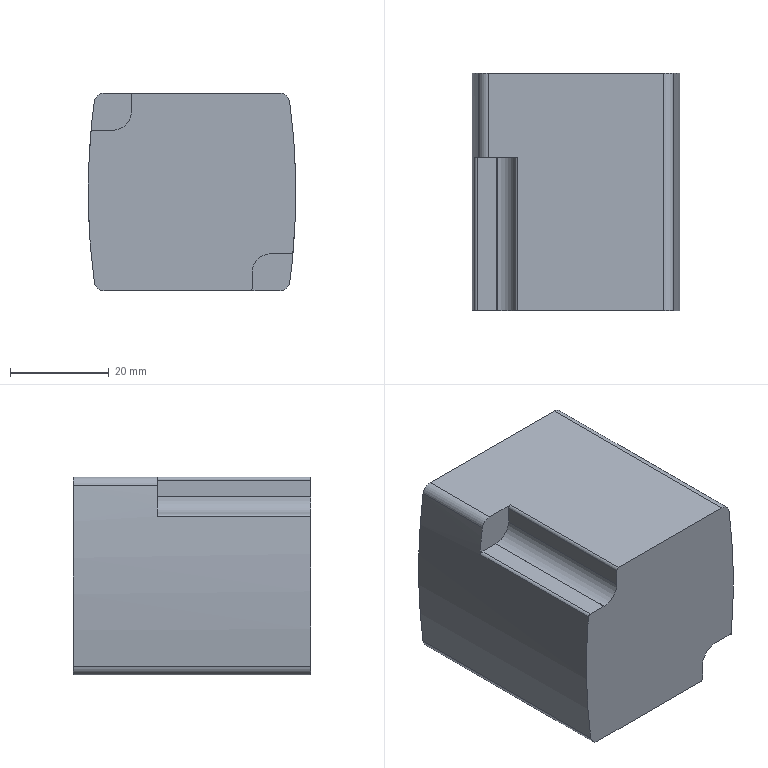Part | SolidWorks | features BaseBody 1 | 1 solid | 27 faces | box 42.009 x 48 x 40 mm | volume 75232 mm3 | cylinder 16 | plane 11 | commonest cylinder face diameters 4 x6 1.2 x5 7.4 x3 268.2 x2
STEP:
#1=CARTESIAN_POINT('',(17.75,48.01,-20.));
#2=VERTEX_POINT('',#1);
#3=CARTESIAN_POINT('',(17.773,48.01,-20.));
#4=VERTEX_POINT('',#3);
#5=CARTESIAN_POINT('',(17.773,48.01,-18.));
#6=DIRECTION('',(0.,-1.,0.));
#7=DIRECTION('',(0.,0.,-1.));
#8=AXIS2_PLACEMENT_3D('',#5,#6,#7);
#9=CIRCLE('',#8,2.);
#10=EDGE_CURVE('',#2,#4,#9,.T.);
#11=ORIENTED_EDGE('',*,*,#10,.T.);
#12=CARTESIAN_POINT('',(17.773,31.01,-20.));
#13=VERTEX_POINT('',#12);
#14=CARTESIAN_POINT('',(17.773,48.01,-20.));
#15=DIRECTION('',(0.,-1.,0.));
#16=VECTOR('',#15,1000.);
#17=LINE('',#14,#16);
#18=EDGE_CURVE('',#4,#13,#17,.T.);
#19=ORIENTED_EDGE('',*,*,#18,.T.);
#20=CARTESIAN_POINT('',(17.75,31.01,-20.));
#21=VERTEX_POINT('',#20);
#22=CARTESIAN_POINT('',(17.773,31.01,-18.));
#23=DIRECTION('',(0.,1.,0.));
#24=DIRECTION('',(0.,0.,-1.));
#25=AXIS2_PLACEMENT_3D('',#22,#23,#24);
#26=CIRCLE('',#25,2.);
#27=EDGE_CURVE('',#13,#21,#26,.T.);
#28=ORIENTED_EDGE('',*,*,#27,.T.);
#29=CARTESIAN_POINT('',(17.75,48.01,-20.));
#30=DIRECTION('',(0.,1.,0.));
#31=VECTOR('',#30,1000.);
#32=LINE('',#29,#31);
#33=EDGE_CURVE('',#21,#2,#32,.T.);
#34=ORIENTED_EDGE('',*,*,#33,.T.);
#35=EDGE_LOOP('',(#11,#19,#28,#34));
#36=FACE_OUTER_BOUND('',#35,.T.);
#37=CARTESIAN_POINT('',(17.773,48.01,-18.));
#38=DIRECTION('',(0.,-1.,0.));
#39=DIRECTION('',(0.,0.,-1.));
#40=AXIS2_PLACEMENT_3D('',#37,#38,#39);
#41=CYLINDRICAL_SURFACE('',#40,2.);
#42=ADVANCED_FACE('',(#36),#41,.T.);
#43=CARTESIAN_POINT('',(-19.75,48.01,-18.3));
#44=VERTEX_POINT('',#43);
#45=CARTESIAN_POINT('',(-17.773,48.01,-20.));
#46=VERTEX_POINT('',#45);
#47=CARTESIAN_POINT('',(-17.773,48.01,-18.));
#48=DIRECTION('',(0.,-1.,0.));
#49=DIRECTION('',(0.,0.,-1.));
#50=AXIS2_PLACEMENT_3D('',#47,#48,#49);
#51=CIRCLE('',#50,2.);
#52=EDGE_CURVE('',#44,#46,#51,.T.);
#53=ORIENTED_EDGE('',*,*,#52,.T.);
#54=CARTESIAN_POINT('',(-17.773,0.01,-20.));
#55=VERTEX_POINT('',#54);
#56=CARTESIAN_POINT('',(-17.773,48.01,-20.));
#57=DIRECTION('',(0.,-1.,0.));
#58=VECTOR('',#57,1000.);
#59=LINE('',#56,#58);
#60=EDGE_CURVE('',#46,#55,#59,.T.);
#61=ORIENTED_EDGE('',*,*,#60,.T.);
#62=CARTESIAN_POINT('',(-19.75,0.01,-18.3));
#63=VERTEX_POINT('',#62);
#64=CARTESIAN_POINT('',(-17.773,0.01,-18.));
#65=DIRECTION('',(0.,1.,0.));
#66=DIRECTION('',(0.,0.,-1.));
#67=AXIS2_PLACEMENT_3D('',#64,#65,#66);
#68=CIRCLE('',#67,2.);
#69=EDGE_CURVE('',#55,#63,#68,.T.);
#70=ORIENTED_EDGE('',*,*,#69,.T.);
#71=CARTESIAN_POINT('',(-19.75,48.01,-18.3));
#72=DIRECTION('',(0.,1.,0.));
#73=VECTOR('',#72,1000.);
#74=LINE('',#71,#73);
#75=EDGE_CURVE('',#63,#44,#74,.T.);
#76=ORIENTED_EDGE('',*,*,#75,.T.);
#77=EDGE_LOOP('',(#53,#61,#70,#76));
#78=FACE_OUTER_BOUND('',#77,.T.);
#79=CARTESIAN_POINT('',(-17.773,48.01,-18.));
#80=DIRECTION('',(0.,-1.,0.));
#81=DIRECTION('',(0.,0.,-1.));
#82=AXIS2_PLACEMENT_3D('',#79,#80,#81);
#83=CYLINDRICAL_SURFACE('',#82,2.);
#84=ADVANCED_FACE('',(#78),#83,.T.);
#85=CARTESIAN_POINT('',(-15.975,31.01,12.51));
#86=VERTEX_POINT('',#85);
#87=CARTESIAN_POINT('',(-12.28,31.01,16.01));
#88=VERTEX_POINT('',#87);
#89=CARTESIAN_POINT('',(-15.975,31.01,16.21));
#90=DIRECTION('',(0.,-1.,0.));
#91=DIRECTION('',(0.,0.,-1.));
#92=AXIS2_PLACEMENT_3D('',#89,#90,#91);
#93=CIRCLE('',#92,3.7);
#94=EDGE_CURVE('',#86,#88,#93,.T.);
#95=ORIENTED_EDGE('',*,*,#94,.F.);
#96=CARTESIAN_POINT('',(-15.975,0.01,12.51));
#97=VERTEX_POINT('',#96);
#98=CARTESIAN_POINT('',(-15.975,31.01,12.51));
#99=DIRECTION('',(0.,-1.,0.));
#100=VECTOR('',#99,1000.);
#101=LINE('',#98,#100);
#102=EDGE_CURVE('',#86,#97,#101,.T.);
#103=ORIENTED_EDGE('',*,*,#102,.T.);
#104=CARTESIAN_POINT('',(-12.28,0.01,16.01));
#105=VERTEX_POINT('',#104);
#106=CARTESIAN_POINT('',(-15.975,0.01,16.21));
#107=DIRECTION('',(0.,1.,0.));
#108=DIRECTION('',(0.,0.,-1.));
#109=AXIS2_PLACEMENT_3D('',#106,#107,#108);
#110=CIRCLE('',#109,3.7);
#111=EDGE_CURVE('',#105,#97,#110,.T.);
#112=ORIENTED_EDGE('',*,*,#111,.F.);
#113=CARTESIAN_POINT('',(-12.28,31.01,16.01));
#114=DIRECTION('',(0.,1.,0.));
#115=VECTOR('',#114,1000.);
#116=LINE('',#113,#115);
#117=EDGE_CURVE('',#105,#88,#116,.T.);
#118=ORIENTED_EDGE('',*,*,#117,.T.);
#119=EDGE_LOOP('',(#95,#103,#112,#118));
#120=FACE_OUTER_BOUND('',#119,.T.);
#121=CARTESIAN_POINT('',(-15.975,31.01,16.21));
#122=DIRECTION('',(0.,-1.,0.));
#123=DIRECTION('',(0.,0.,-1.));
#124=AXIS2_PLACEMENT_3D('',#121,#122,#123);
#125=CYLINDRICAL_SURFACE('',#124,3.7);
#126=ADVANCED_FACE('',(#120),#125,.F.);
#127=CARTESIAN_POINT('',(19.8,31.01,-12.51));
#128=VERTEX_POINT('',#127);
#129=CARTESIAN_POINT('',(19.808,31.01,-12.51));
#130=VERTEX_POINT('',#129);
#131=CARTESIAN_POINT('',(19.808,31.01,-11.91));
#132=DIRECTION('',(0.,-1.,0.));
#133=DIRECTION('',(0.,0.,-1.));
#134=AXIS2_PLACEMENT_3D('',#131,#132,#133);
#135=CIRCLE('',#134,0.6);
#136=EDGE_CURVE('',#128,#130,#135,.T.);
#137=ORIENTED_EDGE('',*,*,#136,.T.);
#138=CARTESIAN_POINT('',(19.808,0.01,-12.51));
#139=VERTEX_POINT('',#138);
#140=CARTESIAN_POINT('',(19.808,31.01,-12.51));
#141=DIRECTION('',(0.,-1.,0.));
#142=VECTOR('',#141,1000.);
#143=LINE('',#140,#142);
#144=EDGE_CURVE('',#130,#139,#143,.T.);
#145=ORIENTED_EDGE('',*,*,#144,.T.);
#146=CARTESIAN_POINT('',(19.8,0.01,-12.51));
#147=VERTEX_POINT('',#146);
#148=CARTESIAN_POINT('',(19.808,0.01,-11.91));
#149=DIRECTION('',(0.,1.,0.));
#150=DIRECTION('',(0.,0.,-1.));
#151=AXIS2_PLACEMENT_3D('',#148,#149,#150);
#152=CIRCLE('',#151,0.6);
#153=EDGE_CURVE('',#139,#147,#152,.T.);
#154=ORIENTED_EDGE('',*,*,#153,.T.);
#155=CARTESIAN_POINT('',(19.8,31.01,-12.51));
#156=DIRECTION('',(0.,1.,0.));
#157=VECTOR('',#156,1000.);
#158=LINE('',#155,#157);
#159=EDGE_CURVE('',#147,#128,#158,.T.);
#160=ORIENTED_EDGE('',*,*,#159,.T.);
#161=EDGE_LOOP('',(#137,#145,#154,#160));
#162=FACE_OUTER_BOUND('',#161,.T.);
#163=CARTESIAN_POINT('',(19.808,31.01,-11.91));
#164=DIRECTION('',(0.,-1.,0.));
#165=DIRECTION('',(0.,0.,-1.));
#166=AXIS2_PLACEMENT_3D('',#163,#164,#165);
#167=CYLINDRICAL_SURFACE('',#166,0.6);
#168=ADVANCED_FACE('',(#162),#167,.T.);
#169=CARTESIAN_POINT('',(19.75,48.01,18.3));
#170=VERTEX_POINT('',#169);
#171=CARTESIAN_POINT('',(17.75,48.01,20.));
#172=VERTEX_POINT('',#171);
#173=CARTESIAN_POINT('',(17.773,48.01,18.));
#174=DIRECTION('',(0.,-1.,0.));
#175=DIRECTION('',(0.,0.,-1.));
#176=AXIS2_PLACEMENT_3D('',#173,#174,#175);
#177=CIRCLE('',#176,2.);
#178=EDGE_CURVE('',#170,#172,#177,.T.);
#179=ORIENTED_EDGE('',*,*,#178,.F.);
#180=CARTESIAN_POINT('',(19.75,48.01,-18.3));
#181=VERTEX_POINT('',#180);
#182=CARTESIAN_POINT('',(-113.095,48.01,0.));
#183=DIRECTION('',(0.,-1.,0.));
#184=DIRECTION('',(0.,0.,-1.));
#185=AXIS2_PLACEMENT_3D('',#182,#183,#184);
#186=CIRCLE('',#185,134.1);
#187=EDGE_CURVE('',#181,#170,#186,.T.);
#188=ORIENTED_EDGE('',*,*,#187,.F.);
#189=CARTESIAN_POINT('',(17.773,48.01,-18.));
#190=DIRECTION('',(0.,-1.,0.));
#191=DIRECTION('',(0.,0.,-1.));
#192=AXIS2_PLACEMENT_3D('',#189,#190,#191);
#193=CIRCLE('',#192,2.);
#194=EDGE_CURVE('',#4,#181,#193,.T.);
#195=ORIENTED_EDGE('',*,*,#194,.F.);
#196=ORIENTED_EDGE('',*,*,#10,.F.);
#197=CARTESIAN_POINT('',(-17.75,48.01,-20.));
#198=VERTEX_POINT('',#197);
#199=CARTESIAN_POINT('',(0.,48.01,-20.));
#200=DIRECTION('',(1.,0.,0.));
#201=VECTOR('',#200,1000.);
#202=LINE('',#199,#201);
#203=EDGE_CURVE('',#198,#2,#202,.T.);
#204=ORIENTED_EDGE('',*,*,#203,.F.);
#205=CARTESIAN_POINT('',(-17.773,48.01,-18.));
#206=DIRECTION('',(0.,-1.,0.));
#207=DIRECTION('',(0.,0.,-1.));
#208=AXIS2_PLACEMENT_3D('',#205,#206,#207);
#209=CIRCLE('',#208,2.);
#210=EDGE_CURVE('',#46,#198,#209,.T.);
#211=ORIENTED_EDGE('',*,*,#210,.F.);
#212=ORIENTED_EDGE('',*,*,#52,.F.);
#213=CARTESIAN_POINT('',(-19.75,48.01,18.3));
#214=VERTEX_POINT('',#213);
#215=CARTESIAN_POINT('',(113.095,48.01,0.));
#216=DIRECTION('',(0.,-1.,0.));
#217=DIRECTION('',(0.,0.,-1.));
#218=AXIS2_PLACEMENT_3D('',#215,#216,#217);
#219=CIRCLE('',#218,134.1);
#220=EDGE_CURVE('',#214,#44,#219,.T.);
#221=ORIENTED_EDGE('',*,*,#220,.F.);
#222=CARTESIAN_POINT('',(-17.75,48.01,20.));
#223=VERTEX_POINT('',#222);
#224=CARTESIAN_POINT('',(-17.773,48.01,18.));
#225=DIRECTION('',(0.,-1.,0.));
#226=DIRECTION('',(0.,0.,-1.));
#227=AXIS2_PLACEMENT_3D('',#224,#225,#226);
#228=CIRCLE('',#227,2.);
#229=EDGE_CURVE('',#223,#214,#228,.T.);
#230=ORIENTED_EDGE('',*,*,#229,.F.);
#231=CARTESIAN_POINT('',(0.,48.01,20.));
#232=DIRECTION('',(-1.,0.,0.));
#233=VECTOR('',#232,1000.);
#234=LINE('',#231,#233);
#235=EDGE_CURVE('',#172,#223,#234,.T.);
#236=ORIENTED_EDGE('',*,*,#235,.F.);
#237=EDGE_LOOP('',(#179,#188,#195,#196,#204,#211,#212,#221,#230,#236));
#238=FACE_OUTER_BOUND('',#237,.T.);
#239=CARTESIAN_POINT('',(0.,48.01,0.));
#240=DIRECTION('',(0.,-1.,0.));
#241=DIRECTION('',(0.,0.,-1.));
#242=AXIS2_PLACEMENT_3D('',#239,#240,#241);
#243=PLANE('',#242);
#244=ADVANCED_FACE('',(#238),#243,.F.);
#245=CARTESIAN_POINT('',(-17.75,31.01,20.));
#246=VERTEX_POINT('',#245);
#247=CARTESIAN_POINT('',(-17.75,48.01,20.));
#248=DIRECTION('',(0.,-1.,0.));
#249=VECTOR('',#248,1000.);
#250=LINE('',#247,#249);
#251=EDGE_CURVE('',#223,#246,#250,.T.);
#252=ORIENTED_EDGE('',*,*,#251,.T.);
#253=CARTESIAN_POINT('',(-11.789,31.01,20.));
#254=VERTEX_POINT('',#253);
#255=CARTESIAN_POINT('',(8.875,31.01,20.));
#256=DIRECTION('',(1.,0.,0.));
#257=VECTOR('',#256,1000.);
#258=LINE('',#255,#257);
#259=EDGE_CURVE('',#246,#254,#258,.T.);
#260=ORIENTED_EDGE('',*,*,#259,.T.);
#261=CARTESIAN_POINT('',(-11.789,0.01,20.));
#262=VERTEX_POINT('',#261);
#263=CARTESIAN_POINT('',(-11.789,48.01,20.));
#264=DIRECTION('',(0.,-1.,0.));
#265=VECTOR('',#264,1000.);
#266=LINE('',#263,#265);
#267=EDGE_CURVE('',#254,#262,#266,.T.);
#268=ORIENTED_EDGE('',*,*,#267,.T.);
#269=CARTESIAN_POINT('',(17.75,0.01,20.));
#270=VERTEX_POINT('',#269);
#271=CARTESIAN_POINT('',(8.875,0.01,20.));
#272=DIRECTION('',(1.,0.,0.));
#273=VECTOR('',#272,1000.);
#274=LINE('',#271,#273);
#275=EDGE_CURVE('',#262,#270,#274,.T.);
#276=ORIENTED_EDGE('',*,*,#275,.T.);
#277=CARTESIAN_POINT('',(17.75,48.01,20.));
#278=DIRECTION('',(0.,1.,0.));
#279=VECTOR('',#278,1000.);
#280=LINE('',#277,#279);
#281=EDGE_CURVE('',#270,#172,#280,.T.);
#282=ORIENTED_EDGE('',*,*,#281,.T.);
#283=ORIENTED_EDGE('',*,*,#235,.T.);
#284=EDGE_LOOP('',(#252,#260,#268,#276,#282,#283));
#285=FACE_OUTER_BOUND('',#284,.T.);
#286=CARTESIAN_POINT('',(8.875,48.01,20.));
#287=DIRECTION('',(0.,0.,1.));
#288=DIRECTION('',(1.,0.,0.));
#289=AXIS2_PLACEMENT_3D('',#286,#287,#288);
#290=PLANE('',#289);
#291=ADVANCED_FACE('',(#285),#290,.T.);
#292=ORIENTED_EDGE('',*,*,#178,.T.);
#293=ORIENTED_EDGE('',*,*,#281,.F.);
#294=CARTESIAN_POINT('',(19.75,0.01,18.3));
#295=VERTEX_POINT('',#294);
#296=CARTESIAN_POINT('',(17.773,0.01,18.));
#297=DIRECTION('',(0.,1.,0.));
#298=DIRECTION('',(0.,0.,-1.));
#299=AXIS2_PLACEMENT_3D('',#296,#297,#298);
#300=CIRCLE('',#299,2.);
#301=EDGE_CURVE('',#270,#295,#300,.T.);
#302=ORIENTED_EDGE('',*,*,#301,.T.);
#303=CARTESIAN_POINT('',(19.75,48.01,18.3));
#304=DIRECTION('',(0.,1.,0.));
#305=VECTOR('',#304,1000.);
#306=LINE('',#303,#305);
#307=EDGE_CURVE('',#295,#170,#306,.T.);
#308=ORIENTED_EDGE('',*,*,#307,.T.);
#309=EDGE_LOOP('',(#292,#293,#302,#308));
#310=FACE_OUTER_BOUND('',#309,.T.);
#311=CARTESIAN_POINT('',(17.773,48.01,18.));
#312=DIRECTION('',(0.,-1.,0.));
#313=DIRECTION('',(0.,0.,-1.));
#314=AXIS2_PLACEMENT_3D('',#311,#312,#313);
#315=CYLINDRICAL_SURFACE('',#314,2.);
#316=ADVANCED_FACE('',(#310),#315,.T.);
#317=ORIENTED_EDGE('',*,*,#307,.F.);
#318=CARTESIAN_POINT('',(20.4,0.01,-12.719));
#319=VERTEX_POINT('',#318);
#320=CARTESIAN_POINT('',(-113.095,0.01,0.));
#321=DIRECTION('',(0.,1.,0.));
#322=DIRECTION('',(0.,0.,-1.));
#323=AXIS2_PLACEMENT_3D('',#320,#321,#322);
#324=CIRCLE('',#323,134.1);
#325=EDGE_CURVE('',#295,#319,#324,.T.);
#326=ORIENTED_EDGE('',*,*,#325,.T.);
#327=CARTESIAN_POINT('',(20.4,31.01,-12.719));
#328=VERTEX_POINT('',#327);
#329=CARTESIAN_POINT('',(20.4,48.01,-12.719));
#330=DIRECTION('',(0.,1.,0.));
#331=VECTOR('',#330,1000.);
#332=LINE('',#329,#331);
#333=EDGE_CURVE('',#319,#328,#332,.T.);
#334=ORIENTED_EDGE('',*,*,#333,.T.);
#335=CARTESIAN_POINT('',(19.75,31.01,-18.3));
#336=VERTEX_POINT('',#335);
#337=CARTESIAN_POINT('',(-113.095,31.01,0.));
#338=DIRECTION('',(0.,1.,0.));
#339=DIRECTION('',(0.,0.,-1.));
#340=AXIS2_PLACEMENT_3D('',#337,#338,#339);
#341=CIRCLE('',#340,134.1);
#342=EDGE_CURVE('',#328,#336,#341,.T.);
#343=ORIENTED_EDGE('',*,*,#342,.T.);
#344=CARTESIAN_POINT('',(19.75,48.01,-18.3));
#345=DIRECTION('',(0.,1.,0.));
#346=VECTOR('',#345,1000.);
#347=LINE('',#344,#346);
#348=EDGE_CURVE('',#336,#181,#347,.T.);
#349=ORIENTED_EDGE('',*,*,#348,.T.);
#350=ORIENTED_EDGE('',*,*,#187,.T.);
#351=EDGE_LOOP('',(#317,#326,#334,#343,#349,#350));
#352=FACE_OUTER_BOUND('',#351,.T.);
#353=CARTESIAN_POINT('',(-113.095,48.01,0.));
#354=DIRECTION('',(0.,-1.,0.));
#355=DIRECTION('',(0.,0.,-1.));
#356=AXIS2_PLACEMENT_3D('',#353,#354,#355);
#357=CYLINDRICAL_SURFACE('',#356,134.1);
#358=ADVANCED_FACE('',(#352),#357,.T.);
#359=ORIENTED_EDGE('',*,*,#18,.F.);
#360=ORIENTED_EDGE('',*,*,#194,.T.);
#361=ORIENTED_EDGE('',*,*,#348,.F.);
#362=CARTESIAN_POINT('',(17.773,31.01,-18.));
#363=DIRECTION('',(0.,1.,0.));
#364=DIRECTION('',(0.,0.,-1.));
#365=AXIS2_PLACEMENT_3D('',#362,#363,#364);
#366=CIRCLE('',#365,2.);
#367=EDGE_CURVE('',#336,#13,#366,.T.);
#368=ORIENTED_EDGE('',*,*,#367,.T.);
#369=EDGE_LOOP('',(#359,#360,#361,#368));
#370=FACE_OUTER_BOUND('',#369,.T.);
#371=CARTESIAN_POINT('',(17.773,48.01,-18.));
#372=DIRECTION('',(0.,-1.,0.));
#373=DIRECTION('',(0.,0.,-1.));
#374=AXIS2_PLACEMENT_3D('',#371,#372,#373);
#375=CYLINDRICAL_SURFACE('',#374,2.);
#376=ADVANCED_FACE('',(#370),#375,.T.);
#377=ORIENTED_EDGE('',*,*,#203,.T.);
#378=ORIENTED_EDGE('',*,*,#33,.F.);
#379=CARTESIAN_POINT('',(11.709,31.01,-20.));
#380=VERTEX_POINT('',#379);
#381=CARTESIAN_POINT('',(0.,31.01,-20.));
#382=DIRECTION('',(-1.,0.,0.));
#383=VECTOR('',#382,1000.);
#384=LINE('',#381,#383);
#385=EDGE_CURVE('',#21,#380,#384,.T.);
#386=ORIENTED_EDGE('',*,*,#385,.T.);
#387=CARTESIAN_POINT('',(11.709,0.01,-20.));
#388=VERTEX_POINT('',#387);
#389=CARTESIAN_POINT('',(11.709,48.01,-20.));
#390=DIRECTION('',(0.,-1.,0.));
#391=VECTOR('',#390,1000.);
#392=LINE('',#389,#391);
#393=EDGE_CURVE('',#380,#388,#392,.T.);
#394=ORIENTED_EDGE('',*,*,#393,.T.);
#395=CARTESIAN_POINT('',(-17.75,0.01,-20.));
#396=VERTEX_POINT('',#395);
#397=CARTESIAN_POINT('',(0.,0.01,-20.));
#398=DIRECTION('',(-1.,0.,0.));
#399=VECTOR('',#398,1000.);
#400=LINE('',#397,#399);
#401=EDGE_CURVE('',#388,#396,#400,.T.);
#402=ORIENTED_EDGE('',*,*,#401,.T.);
#403=CARTESIAN_POINT('',(-17.75,48.01,-20.));
#404=DIRECTION('',(0.,1.,0.));
#405=VECTOR('',#404,1000.);
#406=LINE('',#403,#405);
#407=EDGE_CURVE('',#396,#198,#406,.T.);
#408=ORIENTED_EDGE('',*,*,#407,.T.);
#409=EDGE_LOOP('',(#377,#378,#386,#394,#402,#408));
#410=FACE_OUTER_BOUND('',#409,.T.);
#411=CARTESIAN_POINT('',(0.,48.01,-20.));
#412=DIRECTION('',(0.,0.,-1.));
#413=DIRECTION('',(-1.,0.,0.));
#414=AXIS2_PLACEMENT_3D('',#411,#412,#413);
#415=PLANE('',#414);
#416=ADVANCED_FACE('',(#410),#415,.T.);
#417=ORIENTED_EDGE('',*,*,#60,.F.);
#418=ORIENTED_EDGE('',*,*,#210,.T.);
#419=ORIENTED_EDGE('',*,*,#407,.F.);
#420=CARTESIAN_POINT('',(-17.773,0.01,-18.));
#421=DIRECTION('',(0.,1.,0.));
#422=DIRECTION('',(0.,0.,-1.));
#423=AXIS2_PLACEMENT_3D('',#420,#421,#422);
#424=CIRCLE('',#423,2.);
#425=EDGE_CURVE('',#396,#55,#424,.T.);
#426=ORIENTED_EDGE('',*,*,#425,.T.);
#427=EDGE_LOOP('',(#417,#418,#419,#426));
#428=FACE_OUTER_BOUND('',#427,.T.);
#429=CARTESIAN_POINT('',(-17.773,48.01,-18.));
#430=DIRECTION('',(0.,-1.,0.));
#431=DIRECTION('',(0.,0.,-1.));
#432=AXIS2_PLACEMENT_3D('',#429,#430,#431);
#433=CYLINDRICAL_SURFACE('',#432,2.);
#434=ADVANCED_FACE('',(#428),#433,.T.);
#435=CARTESIAN_POINT('',(-20.458,0.01,12.1));
#436=VERTEX_POINT('',#435);
#437=CARTESIAN_POINT('',(113.095,0.01,0.));
#438=DIRECTION('',(0.,1.,0.));
#439=DIRECTION('',(0.,0.,-1.));
#440=AXIS2_PLACEMENT_3D('',#437,#438,#439);
#441=CIRCLE('',#440,134.1);
#442=EDGE_CURVE('',#63,#436,#441,.T.);
#443=ORIENTED_EDGE('',*,*,#442,.T.);
#444=CARTESIAN_POINT('',(-20.458,31.01,12.1));
#445=VERTEX_POINT('',#444);
#446=CARTESIAN_POINT('',(-20.458,48.01,12.1));
#447=DIRECTION('',(0.,1.,0.));
#448=VECTOR('',#447,1000.);
#449=LINE('',#446,#448);
#450=EDGE_CURVE('',#436,#445,#449,.T.);
#451=ORIENTED_EDGE('',*,*,#450,.T.);
#452=CARTESIAN_POINT('',(-19.75,31.01,18.3));
#453=VERTEX_POINT('',#452);
#454=CARTESIAN_POINT('',(113.095,31.01,0.));
#455=DIRECTION('',(0.,1.,0.));
#456=DIRECTION('',(0.,0.,-1.));
#457=AXIS2_PLACEMENT_3D('',#454,#455,#456);
#458=CIRCLE('',#457,134.1);
#459=EDGE_CURVE('',#445,#453,#458,.T.);
#460=ORIENTED_EDGE('',*,*,#459,.T.);
#461=CARTESIAN_POINT('',(-19.75,48.01,18.3));
#462=DIRECTION('',(0.,1.,0.));
#463=VECTOR('',#462,1000.);
#464=LINE('',#461,#463);
#465=EDGE_CURVE('',#453,#214,#464,.T.);
#466=ORIENTED_EDGE('',*,*,#465,.T.);
#467=ORIENTED_EDGE('',*,*,#220,.T.);
#468=ORIENTED_EDGE('',*,*,#75,.F.);
#469=EDGE_LOOP('',(#443,#451,#460,#466,#467,#468));
#470=FACE_OUTER_BOUND('',#469,.T.);
#471=CARTESIAN_POINT('',(113.095,48.01,0.));
#472=DIRECTION('',(0.,-1.,0.));
#473=DIRECTION('',(0.,0.,-1.));
#474=AXIS2_PLACEMENT_3D('',#471,#472,#473);
#475=CYLINDRICAL_SURFACE('',#474,134.1);
#476=ADVANCED_FACE('',(#470),#475,.T.);
#477=ORIENTED_EDGE('',*,*,#229,.T.);
#478=ORIENTED_EDGE('',*,*,#465,.F.);
#479=CARTESIAN_POINT('',(-17.773,31.01,18.));
#480=DIRECTION('',(0.,1.,0.));
#481=DIRECTION('',(0.,0.,-1.));
#482=AXIS2_PLACEMENT_3D('',#479,#480,#481);
#483=CIRCLE('',#482,2.);
#484=EDGE_CURVE('',#453,#246,#483,.T.);
#485=ORIENTED_EDGE('',*,*,#484,.T.);
#486=ORIENTED_EDGE('',*,*,#251,.F.);
#487=EDGE_LOOP('',(#477,#478,#485,#486));
#488=FACE_OUTER_BOUND('',#487,.T.);
#489=CARTESIAN_POINT('',(-17.773,48.01,18.));
#490=DIRECTION('',(0.,-1.,0.));
#491=DIRECTION('',(0.,0.,-1.));
#492=AXIS2_PLACEMENT_3D('',#489,#490,#491);
#493=CYLINDRICAL_SURFACE('',#492,2.);
#494=ADVANCED_FACE('',(#488),#493,.T.);
#495=CARTESIAN_POINT('',(-12.28,31.01,19.41));
#496=VERTEX_POINT('',#495);
#497=CARTESIAN_POINT('',(-12.28,31.01,16.501));
#498=DIRECTION('',(0.,0.,1.));
#499=VECTOR('',#498,1000.);
#500=LINE('',#497,#499);
#501=EDGE_CURVE('',#88,#496,#500,.T.);
#502=ORIENTED_EDGE('',*,*,#501,.T.);
#503=CARTESIAN_POINT('',(-11.68,31.01,19.41));
#504=DIRECTION('',(0.,1.,0.));
#505=DIRECTION('',(0.,0.,-1.));
#506=AXIS2_PLACEMENT_3D('',#503,#504,#505);
#507=CIRCLE('',#506,0.6);
#508=EDGE_CURVE('',#496,#254,#507,.T.);
#509=ORIENTED_EDGE('',*,*,#508,.T.);
#510=ORIENTED_EDGE('',*,*,#259,.F.);
#511=ORIENTED_EDGE('',*,*,#484,.F.);
#512=ORIENTED_EDGE('',*,*,#459,.F.);
#513=CARTESIAN_POINT('',(-19.88,31.01,12.51));
#514=VERTEX_POINT('',#513);
#515=CARTESIAN_POINT('',(-19.888,31.01,11.91));
#516=DIRECTION('',(0.,1.,0.));
#517=DIRECTION('',(0.,0.,-1.));
#518=AXIS2_PLACEMENT_3D('',#515,#516,#517);
#519=CIRCLE('',#518,0.6);
#520=EDGE_CURVE('',#445,#514,#519,.T.);
#521=ORIENTED_EDGE('',*,*,#520,.T.);
#522=CARTESIAN_POINT('',(-15.98,31.01,12.51));
#523=VERTEX_POINT('',#522);
#524=CARTESIAN_POINT('',(-16.586,31.01,12.51));
#525=DIRECTION('',(1.,0.,0.));
#526=VECTOR('',#525,1000.);
#527=LINE('',#524,#526);
#528=EDGE_CURVE('',#514,#523,#527,.T.);
#529=ORIENTED_EDGE('',*,*,#528,.T.);
#530=CARTESIAN_POINT('',(-15.975,31.01,16.21));
#531=DIRECTION('',(0.,-1.,0.));
#532=DIRECTION('',(0.,0.,-1.));
#533=AXIS2_PLACEMENT_3D('',#530,#531,#532);
#534=CIRCLE('',#533,3.7);
#535=EDGE_CURVE('',#523,#86,#534,.T.);
#536=ORIENTED_EDGE('',*,*,#535,.T.);
#537=ORIENTED_EDGE('',*,*,#94,.T.);
#538=EDGE_LOOP('',(#502,#509,#510,#511,#512,#521,#529,#536,#537));
#539=FACE_OUTER_BOUND('',#538,.T.);
#540=CARTESIAN_POINT('',(-16.586,31.01,16.501));
#541=DIRECTION('',(0.,-1.,0.));
#542=DIRECTION('',(0.,0.,-1.));
#543=AXIS2_PLACEMENT_3D('',#540,#541,#542);
#544=PLANE('',#543);
#545=ADVANCED_FACE('',(#539),#544,.T.);
#546=CARTESIAN_POINT('',(15.9,0.01,-12.51));
#547=VERTEX_POINT('',#546);
#548=CARTESIAN_POINT('',(0.,0.01,-12.51));
#549=DIRECTION('',(1.,0.,0.));
#550=VECTOR('',#549,1000.);
#551=LINE('',#548,#550);
#552=EDGE_CURVE('',#547,#147,#551,.T.);
#553=ORIENTED_EDGE('',*,*,#552,.T.);
#554=ORIENTED_EDGE('',*,*,#153,.F.);
#555=CARTESIAN_POINT('',(20.4,0.01,-12.01));
#556=VERTEX_POINT('',#555);
#557=CARTESIAN_POINT('',(19.808,0.01,-11.91));
#558=DIRECTION('',(0.,1.,0.));
#559=DIRECTION('',(0.,0.,-1.));
#560=AXIS2_PLACEMENT_3D('',#557,#558,#559);
#561=CIRCLE('',#560,0.6);
#562=EDGE_CURVE('',#556,#139,#561,.T.);
#563=ORIENTED_EDGE('',*,*,#562,.F.);
#564=CARTESIAN_POINT('',(20.4,0.01,0.));
#565=DIRECTION('',(0.,0.,-1.));
#566=VECTOR('',#565,1000.);
#567=LINE('',#564,#566);
#568=EDGE_CURVE('',#556,#319,#567,.T.);
#569=ORIENTED_EDGE('',*,*,#568,.T.);
#570=ORIENTED_EDGE('',*,*,#325,.F.);
#571=ORIENTED_EDGE('',*,*,#301,.F.);
#572=ORIENTED_EDGE('',*,*,#275,.F.);
#573=CARTESIAN_POINT('',(-12.28,0.01,19.41));
#574=VERTEX_POINT('',#573);
#575=CARTESIAN_POINT('',(-11.68,0.01,19.41));
#576=DIRECTION('',(0.,-1.,0.));
#577=DIRECTION('',(0.,0.,-1.));
#578=AXIS2_PLACEMENT_3D('',#575,#576,#577);
#579=CIRCLE('',#578,0.6);
#580=EDGE_CURVE('',#262,#574,#579,.T.);
#581=ORIENTED_EDGE('',*,*,#580,.T.);
#582=CARTESIAN_POINT('',(-12.28,0.01,0.));
#583=DIRECTION('',(0.,0.,-1.));
#584=VECTOR('',#583,1000.);
#585=LINE('',#582,#584);
#586=EDGE_CURVE('',#574,#105,#585,.T.);
#587=ORIENTED_EDGE('',*,*,#586,.T.);
#588=ORIENTED_EDGE('',*,*,#111,.T.);
#589=CARTESIAN_POINT('',(-15.98,0.01,12.51));
#590=VERTEX_POINT('',#589);
#591=CARTESIAN_POINT('',(-15.975,0.01,16.21));
#592=DIRECTION('',(0.,1.,0.));
#593=DIRECTION('',(0.,0.,-1.));
#594=AXIS2_PLACEMENT_3D('',#591,#592,#593);
#595=CIRCLE('',#594,3.7);
#596=EDGE_CURVE('',#97,#590,#595,.T.);
#597=ORIENTED_EDGE('',*,*,#596,.T.);
#598=CARTESIAN_POINT('',(-19.88,0.01,12.51));
#599=VERTEX_POINT('',#598);
#600=CARTESIAN_POINT('',(0.,0.01,12.51));
#601=DIRECTION('',(-1.,0.,0.));
#602=VECTOR('',#601,1000.);
#603=LINE('',#600,#602);
#604=EDGE_CURVE('',#590,#599,#603,.T.);
#605=ORIENTED_EDGE('',*,*,#604,.T.);
#606=CARTESIAN_POINT('',(-19.888,0.01,11.91));
#607=DIRECTION('',(0.,-1.,0.));
#608=DIRECTION('',(0.,0.,-1.));
#609=AXIS2_PLACEMENT_3D('',#606,#607,#608);
#610=CIRCLE('',#609,0.6);
#611=EDGE_CURVE('',#599,#436,#610,.T.);
#612=ORIENTED_EDGE('',*,*,#611,.T.);
#613=ORIENTED_EDGE('',*,*,#442,.F.);
#614=ORIENTED_EDGE('',*,*,#69,.F.);
#615=ORIENTED_EDGE('',*,*,#425,.F.);
#616=ORIENTED_EDGE('',*,*,#401,.F.);
#617=CARTESIAN_POINT('',(12.2,0.01,-19.41));
#618=VERTEX_POINT('',#617);
#619=CARTESIAN_POINT('',(11.6,0.01,-19.41));
#620=DIRECTION('',(0.,-1.,0.));
#621=DIRECTION('',(0.,0.,-1.));
#622=AXIS2_PLACEMENT_3D('',#619,#620,#621);
#623=CIRCLE('',#622,0.6);
#624=EDGE_CURVE('',#388,#618,#623,.T.);
#625=ORIENTED_EDGE('',*,*,#624,.T.);
#626=CARTESIAN_POINT('',(12.2,0.01,-16.01));
#627=VERTEX_POINT('',#626);
#628=CARTESIAN_POINT('',(12.2,0.01,0.));
#629=DIRECTION('',(0.,0.,1.));
#630=VECTOR('',#629,1000.);
#631=LINE('',#628,#630);
#632=EDGE_CURVE('',#618,#627,#631,.T.);
#633=ORIENTED_EDGE('',*,*,#632,.T.);
#634=CARTESIAN_POINT('',(15.895,0.01,-16.21));
#635=DIRECTION('',(0.,1.,0.));
#636=DIRECTION('',(0.,0.,-1.));
#637=AXIS2_PLACEMENT_3D('',#634,#635,#636);
#638=CIRCLE('',#637,3.7);
#639=EDGE_CURVE('',#627,#547,#638,.T.);
#640=ORIENTED_EDGE('',*,*,#639,.T.);
#641=EDGE_LOOP('',(#553,#554,#563,#569,#570,#571,#572,#581,#587,#588,#597,#605,#612,#613,#614,#615,#616,#625,#633,#640));
#642=FACE_OUTER_BOUND('',#641,.T.);
#643=CARTESIAN_POINT('',(0.,0.01,0.));
#644=DIRECTION('',(0.,-1.,0.));
#645=DIRECTION('',(0.,0.,-1.));
#646=AXIS2_PLACEMENT_3D('',#643,#644,#645);
#647=PLANE('',#646);
#648=ADVANCED_FACE('',(#642),#647,.T.);
#649=CARTESIAN_POINT('',(-12.28,31.01,19.41));
#650=DIRECTION('',(0.,-1.,0.));
#651=VECTOR('',#650,1000.);
#652=LINE('',#649,#651);
#653=EDGE_CURVE('',#496,#574,#652,.T.);
#654=ORIENTED_EDGE('',*,*,#653,.T.);
#655=ORIENTED_EDGE('',*,*,#580,.F.);
#656=ORIENTED_EDGE('',*,*,#267,.F.);
#657=ORIENTED_EDGE('',*,*,#508,.F.);
#658=EDGE_LOOP('',(#654,#655,#656,#657));
#659=FACE_OUTER_BOUND('',#658,.T.);
#660=CARTESIAN_POINT('',(-11.68,31.01,19.41));
#661=DIRECTION('',(0.,-1.,0.));
#662=DIRECTION('',(0.,0.,-1.));
#663=AXIS2_PLACEMENT_3D('',#660,#661,#662);
#664=CYLINDRICAL_SURFACE('',#663,0.6);
#665=ADVANCED_FACE('',(#659),#664,.T.);
#666=ORIENTED_EDGE('',*,*,#385,.F.);
#667=ORIENTED_EDGE('',*,*,#27,.F.);
#668=ORIENTED_EDGE('',*,*,#367,.F.);
#669=ORIENTED_EDGE('',*,*,#342,.F.);
#670=CARTESIAN_POINT('',(20.4,31.01,-12.01));
#671=VERTEX_POINT('',#670);
#672=CARTESIAN_POINT('',(20.4,31.01,-16.501));
#673=DIRECTION('',(0.,0.,1.));
#674=VECTOR('',#673,1000.);
#675=LINE('',#672,#674);
#676=EDGE_CURVE('',#328,#671,#675,.T.);
#677=ORIENTED_EDGE('',*,*,#676,.T.);
#678=CARTESIAN_POINT('',(19.808,31.01,-11.91));
#679=DIRECTION('',(0.,-1.,0.));
#680=DIRECTION('',(0.,0.,-1.));
#681=AXIS2_PLACEMENT_3D('',#678,#679,#680);
#682=CIRCLE('',#681,0.6);
#683=EDGE_CURVE('',#130,#671,#682,.T.);
#684=ORIENTED_EDGE('',*,*,#683,.F.);
#685=ORIENTED_EDGE('',*,*,#136,.F.);
#686=CARTESIAN_POINT('',(15.9,31.01,-12.51));
#687=VERTEX_POINT('',#686);
#688=CARTESIAN_POINT('',(16.506,31.01,-12.51));
#689=DIRECTION('',(-1.,0.,0.));
#690=VECTOR('',#689,1000.);
#691=LINE('',#688,#690);
#692=EDGE_CURVE('',#128,#687,#691,.T.);
#693=ORIENTED_EDGE('',*,*,#692,.T.);
#694=CARTESIAN_POINT('',(12.2,31.01,-16.01));
#695=VERTEX_POINT('',#694);
#696=CARTESIAN_POINT('',(15.895,31.01,-16.21));
#697=DIRECTION('',(0.,-1.,0.));
#698=DIRECTION('',(0.,0.,-1.));
#699=AXIS2_PLACEMENT_3D('',#696,#697,#698);
#700=CIRCLE('',#699,3.7);
#701=EDGE_CURVE('',#687,#695,#700,.T.);
#702=ORIENTED_EDGE('',*,*,#701,.T.);
#703=CARTESIAN_POINT('',(12.2,31.01,-19.41));
#704=VERTEX_POINT('',#703);
#705=CARTESIAN_POINT('',(12.2,31.01,-16.501));
#706=DIRECTION('',(0.,0.,-1.));
#707=VECTOR('',#706,1000.);
#708=LINE('',#705,#707);
#709=EDGE_CURVE('',#695,#704,#708,.T.);
#710=ORIENTED_EDGE('',*,*,#709,.T.);
#711=CARTESIAN_POINT('',(11.6,31.01,-19.41));
#712=DIRECTION('',(0.,1.,0.));
#713=DIRECTION('',(0.,0.,-1.));
#714=AXIS2_PLACEMENT_3D('',#711,#712,#713);
#715=CIRCLE('',#714,0.6);
#716=EDGE_CURVE('',#704,#380,#715,.T.);
#717=ORIENTED_EDGE('',*,*,#716,.T.);
#718=EDGE_LOOP('',(#666,#667,#668,#669,#677,#684,#685,#693,#702,#710,#717));
#719=FACE_OUTER_BOUND('',#718,.T.);
#720=CARTESIAN_POINT('',(16.506,31.01,-16.501));
#721=DIRECTION('',(0.,-1.,0.));
#722=DIRECTION('',(0.,0.,-1.));
#723=AXIS2_PLACEMENT_3D('',#720,#721,#722);
#724=PLANE('',#723);
#725=ADVANCED_FACE('',(#719),#724,.T.);
#726=ORIENTED_EDGE('',*,*,#568,.F.);
#727=CARTESIAN_POINT('',(20.4,31.01,-12.01));
#728=DIRECTION('',(0.,-1.,0.));
#729=VECTOR('',#728,1000.);
#730=LINE('',#727,#729);
#731=EDGE_CURVE('',#671,#556,#730,.T.);
#732=ORIENTED_EDGE('',*,*,#731,.F.);
#733=ORIENTED_EDGE('',*,*,#676,.F.);
#734=ORIENTED_EDGE('',*,*,#333,.F.);
#735=EDGE_LOOP('',(#726,#732,#733,#734));
#736=FACE_OUTER_BOUND('',#735,.T.);
#737=CARTESIAN_POINT('',(20.4,31.01,-16.01));
#738=DIRECTION('',(1.,0.,0.));
#739=DIRECTION('',(0.,0.,-1.));
#740=AXIS2_PLACEMENT_3D('',#737,#738,#739);
#741=PLANE('',#740);
#742=ADVANCED_FACE('',(#736),#741,.F.);
#743=CARTESIAN_POINT('',(12.2,31.01,-19.41));
#744=DIRECTION('',(0.,-1.,0.));
#745=VECTOR('',#744,1000.);
#746=LINE('',#743,#745);
#747=EDGE_CURVE('',#704,#618,#746,.T.);
#748=ORIENTED_EDGE('',*,*,#747,.T.);
#749=ORIENTED_EDGE('',*,*,#624,.F.);
#750=ORIENTED_EDGE('',*,*,#393,.F.);
#751=ORIENTED_EDGE('',*,*,#716,.F.);
#752=EDGE_LOOP('',(#748,#749,#750,#751));
#753=FACE_OUTER_BOUND('',#752,.T.);
#754=CARTESIAN_POINT('',(11.6,31.01,-19.41));
#755=DIRECTION('',(0.,-1.,0.));
#756=DIRECTION('',(0.,0.,-1.));
#757=AXIS2_PLACEMENT_3D('',#754,#755,#756);
#758=CYLINDRICAL_SURFACE('',#757,0.6);
#759=ADVANCED_FACE('',(#753),#758,.T.);
#760=CARTESIAN_POINT('',(-19.88,31.01,12.51));
#761=DIRECTION('',(0.,1.,0.));
#762=VECTOR('',#761,1000.);
#763=LINE('',#760,#762);
#764=EDGE_CURVE('',#599,#514,#763,.T.);
#765=ORIENTED_EDGE('',*,*,#764,.T.);
#766=ORIENTED_EDGE('',*,*,#520,.F.);
#767=ORIENTED_EDGE('',*,*,#450,.F.);
#768=ORIENTED_EDGE('',*,*,#611,.F.);
#769=EDGE_LOOP('',(#765,#766,#767,#768));
#770=FACE_OUTER_BOUND('',#769,.T.);
#771=CARTESIAN_POINT('',(-19.888,31.01,11.91));
#772=DIRECTION('',(0.,-1.,0.));
#773=DIRECTION('',(0.,0.,-1.));
#774=AXIS2_PLACEMENT_3D('',#771,#772,#773);
#775=CYLINDRICAL_SURFACE('',#774,0.6);
#776=ADVANCED_FACE('',(#770),#775,.T.);
#777=ORIENTED_EDGE('',*,*,#653,.F.);
#778=ORIENTED_EDGE('',*,*,#501,.F.);
#779=ORIENTED_EDGE('',*,*,#117,.F.);
#780=ORIENTED_EDGE('',*,*,#586,.F.);
#781=EDGE_LOOP('',(#777,#778,#779,#780));
#782=FACE_OUTER_BOUND('',#781,.T.);
#783=CARTESIAN_POINT('',(-12.28,31.01,17.71));
#784=DIRECTION('',(1.,0.,0.));
#785=DIRECTION('',(0.,0.,-1.));
#786=AXIS2_PLACEMENT_3D('',#783,#784,#785);
#787=PLANE('',#786);
#788=ADVANCED_FACE('',(#782),#787,.F.);
#789=ORIENTED_EDGE('',*,*,#102,.F.);
#790=ORIENTED_EDGE('',*,*,#535,.F.);
#791=CARTESIAN_POINT('',(-15.98,31.01,12.51));
#792=DIRECTION('',(0.,1.,0.));
#793=VECTOR('',#792,1000.);
#794=LINE('',#791,#793);
#795=EDGE_CURVE('',#590,#523,#794,.T.);
#796=ORIENTED_EDGE('',*,*,#795,.F.);
#797=ORIENTED_EDGE('',*,*,#596,.F.);
#798=EDGE_LOOP('',(#789,#790,#796,#797));
#799=FACE_OUTER_BOUND('',#798,.T.);
#800=CARTESIAN_POINT('',(-15.975,31.01,16.21));
#801=DIRECTION('',(0.,-1.,0.));
#802=DIRECTION('',(0.,0.,-1.));
#803=AXIS2_PLACEMENT_3D('',#800,#801,#802);
#804=CYLINDRICAL_SURFACE('',#803,3.7);
#805=ADVANCED_FACE('',(#799),#804,.F.);
#806=ORIENTED_EDGE('',*,*,#795,.T.);
#807=ORIENTED_EDGE('',*,*,#528,.F.);
#808=ORIENTED_EDGE('',*,*,#764,.F.);
#809=ORIENTED_EDGE('',*,*,#604,.F.);
#810=EDGE_LOOP('',(#806,#807,#808,#809));
#811=FACE_OUTER_BOUND('',#810,.T.);
#812=CARTESIAN_POINT('',(-17.93,31.01,12.51));
#813=DIRECTION('',(0.,0.,-1.));
#814=DIRECTION('',(-1.,0.,0.));
#815=AXIS2_PLACEMENT_3D('',#812,#813,#814);
#816=PLANE('',#815);
#817=ADVANCED_FACE('',(#811),#816,.F.);
#818=CARTESIAN_POINT('',(15.9,31.01,-12.51));
#819=DIRECTION('',(0.,-1.,0.));
#820=VECTOR('',#819,1000.);
#821=LINE('',#818,#820);
#822=EDGE_CURVE('',#687,#547,#821,.T.);
#823=ORIENTED_EDGE('',*,*,#822,.F.);
#824=ORIENTED_EDGE('',*,*,#692,.F.);
#825=ORIENTED_EDGE('',*,*,#159,.F.);
#826=ORIENTED_EDGE('',*,*,#552,.F.);
#827=EDGE_LOOP('',(#823,#824,#825,#826));
#828=FACE_OUTER_BOUND('',#827,.T.);
#829=CARTESIAN_POINT('',(17.85,31.01,-12.51));
#830=DIRECTION('',(0.,0.,1.));
#831=DIRECTION('',(1.,0.,0.));
#832=AXIS2_PLACEMENT_3D('',#829,#830,#831);
#833=PLANE('',#832);
#834=ADVANCED_FACE('',(#828),#833,.F.);
#835=CARTESIAN_POINT('',(12.2,31.01,-16.01));
#836=DIRECTION('',(0.,-1.,0.));
#837=VECTOR('',#836,1000.);
#838=LINE('',#835,#837);
#839=EDGE_CURVE('',#695,#627,#838,.T.);
#840=ORIENTED_EDGE('',*,*,#839,.F.);
#841=ORIENTED_EDGE('',*,*,#701,.F.);
#842=ORIENTED_EDGE('',*,*,#822,.T.);
#843=ORIENTED_EDGE('',*,*,#639,.F.);
#844=EDGE_LOOP('',(#840,#841,#842,#843));
#845=FACE_OUTER_BOUND('',#844,.T.);
#846=CARTESIAN_POINT('',(15.895,31.01,-16.21));
#847=DIRECTION('',(0.,-1.,0.));
#848=DIRECTION('',(0.,0.,-1.));
#849=AXIS2_PLACEMENT_3D('',#846,#847,#848);
#850=CYLINDRICAL_SURFACE('',#849,3.7);
#851=ADVANCED_FACE('',(#845),#850,.F.);
#852=ORIENTED_EDGE('',*,*,#747,.F.);
#853=ORIENTED_EDGE('',*,*,#709,.F.);
#854=ORIENTED_EDGE('',*,*,#839,.T.);
#855=ORIENTED_EDGE('',*,*,#632,.F.);
#856=EDGE_LOOP('',(#852,#853,#854,#855));
#857=FACE_OUTER_BOUND('',#856,.T.);
#858=CARTESIAN_POINT('',(12.2,31.01,-17.71));
#859=DIRECTION('',(-1.,0.,0.));
#860=DIRECTION('',(0.,0.,1.));
#861=AXIS2_PLACEMENT_3D('',#858,#859,#860);
#862=PLANE('',#861);
#863=ADVANCED_FACE('',(#857),#862,.F.);
#864=ORIENTED_EDGE('',*,*,#144,.F.);
#865=ORIENTED_EDGE('',*,*,#683,.T.);
#866=ORIENTED_EDGE('',*,*,#731,.T.);
#867=ORIENTED_EDGE('',*,*,#562,.T.);
#868=EDGE_LOOP('',(#864,#865,#866,#867));
#869=FACE_OUTER_BOUND('',#868,.T.);
#870=CARTESIAN_POINT('',(19.808,31.01,-11.91));
#871=DIRECTION('',(0.,-1.,0.));
#872=DIRECTION('',(0.,0.,-1.));
#873=AXIS2_PLACEMENT_3D('',#870,#871,#872);
#874=CYLINDRICAL_SURFACE('',#873,0.6);
#875=ADVANCED_FACE('',(#869),#874,.T.);
#876=CLOSED_SHELL('',(#42,#84,#126,#168,#244,#291,#316,#358,#376,#416,#434,#476,#494,#545,#648,#665,#725,#742,#759,#776,#788,#805,#817,#834,#851,#863,#875));
#877=MANIFOLD_SOLID_BREP('',#876);
#878=CARTESIAN_POINT('',(0.,0.,0.));
#879=DIRECTION('',(0.,0.,1.));
#880=DIRECTION('',(1.,0.,0.));
#881=AXIS2_PLACEMENT_3D('',#878,#879,#880);
#882=(LENGTH_UNIT()NAMED_UNIT(*)SI_UNIT(.MILLI.,.METRE.));
#883=UNCERTAINTY_MEASURE_WITH_UNIT(LENGTH_MEASURE(0.00001),#882,'','');
#884=(NAMED_UNIT(*)PLANE_ANGLE_UNIT()SI_UNIT($,.RADIAN.));
#885=(NAMED_UNIT(*)SI_UNIT($,.STERADIAN.)SOLID_ANGLE_UNIT());
#886=(GEOMETRIC_REPRESENTATION_CONTEXT(3)GLOBAL_UNCERTAINTY_ASSIGNED_CONTEXT((#883))GLOBAL_UNIT_ASSIGNED_CONTEXT((#882,#884,#885))REPRESENTATION_CONTEXT('',''));
#887=ADVANCED_BREP_SHAPE_REPRESENTATION('',(#877,#881),#886);